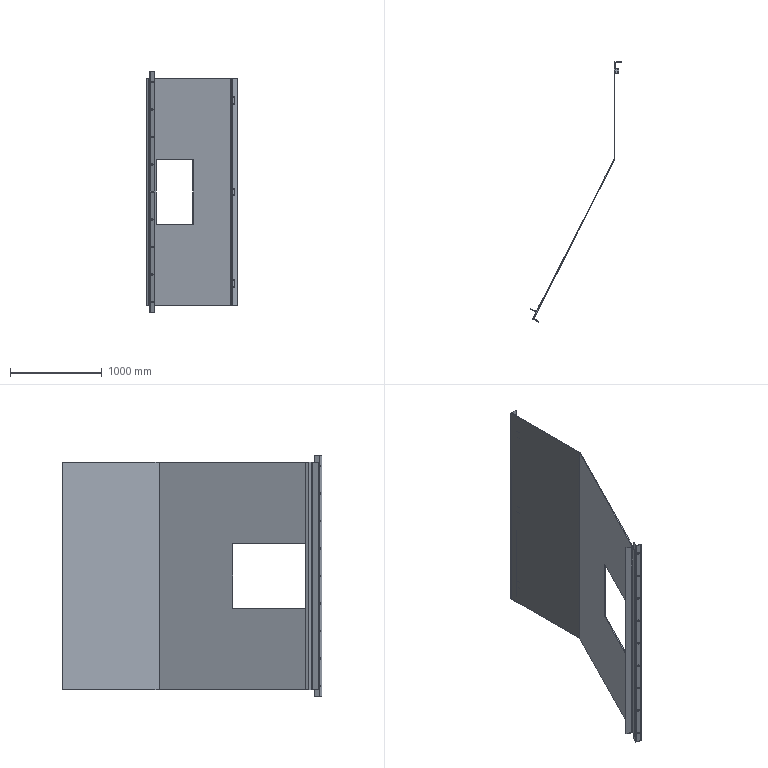Part | STEP file | Upper hopper rear baffle_Default<As machined> | 7 solids | 113 faces | box 1001 x 2838 x 2626 mm | volume 60427980 mm3 | plane 70 | cylinder 43 | commonest cylinder face diameters 18 x20 3.333 x8 8 x6 16 x6 4 x1 14 x1